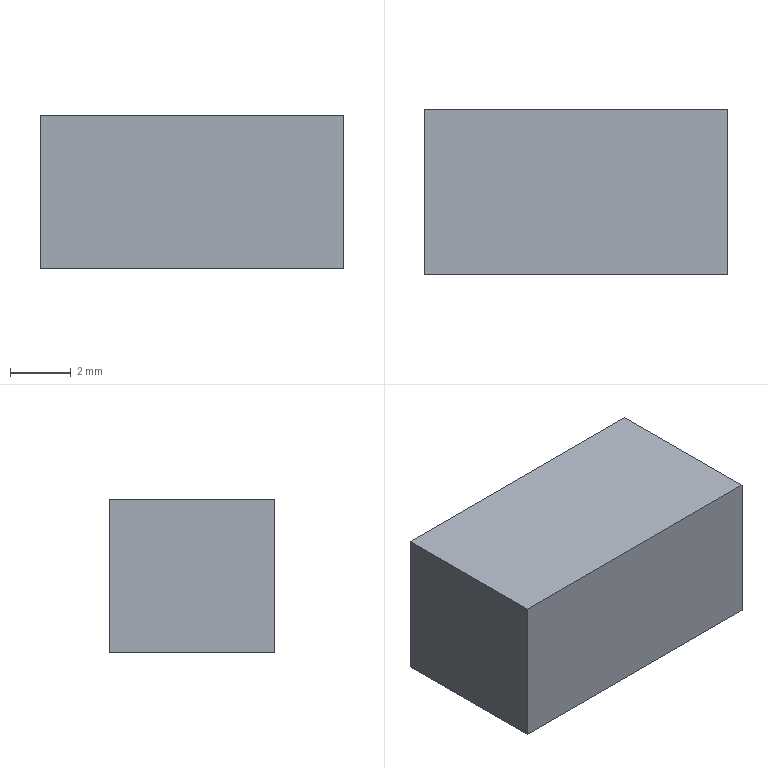Part | NX | features solid 2 | 1 solid | 6 faces | box 10 x 5.446 x 5.048 mm | volume 274.878 mm3 | plane 6
STEP:
#1=CARTESIAN_POINT('',(2250.,364.446,-670.));
#2=VERTEX_POINT('',#1);
#3=CARTESIAN_POINT('',(2250.,359.,-670.));
#4=VERTEX_POINT('',#3);
#5=CARTESIAN_POINT('',(2250.,364.446,-670.));
#6=CARTESIAN_POINT('',(2250.,362.63,-670.));
#7=CARTESIAN_POINT('',(2250.,360.815,-670.));
#8=CARTESIAN_POINT('',(2250.,359.,-670.));
#9=B_SPLINE_CURVE_WITH_KNOTS('',3,(#5,#6,#7,#8),.UNSPECIFIED.,.F.,.F.,(4,4),(0.,0.2595),.PIECEWISE_BEZIER_KNOTS.);
#10=EDGE_CURVE('',#2,#4,#9,.T.);
#11=ORIENTED_EDGE('',*,*,#10,.F.);
#12=CARTESIAN_POINT('',(2260.,364.446,-670.));
#13=VERTEX_POINT('',#12);
#14=CARTESIAN_POINT('',(2260.,364.446,-670.));
#15=DIRECTION('',(-1.,0.,0.));
#16=VECTOR('',#15,1000.);
#17=LINE('',#14,#16);
#18=EDGE_CURVE('',#13,#2,#17,.T.);
#19=ORIENTED_EDGE('',*,*,#18,.F.);
#20=CARTESIAN_POINT('',(2260.,359.,-670.));
#21=VERTEX_POINT('',#20);
#22=CARTESIAN_POINT('',(2260.,364.446,-670.));
#23=CARTESIAN_POINT('',(2260.,362.63,-670.));
#24=CARTESIAN_POINT('',(2260.,360.815,-670.));
#25=CARTESIAN_POINT('',(2260.,359.,-670.));
#26=B_SPLINE_CURVE_WITH_KNOTS('',3,(#22,#23,#24,#25),.UNSPECIFIED.,.F.,.F.,(4,4),(0.,0.2595),.PIECEWISE_BEZIER_KNOTS.);
#27=EDGE_CURVE('',#13,#21,#26,.T.);
#28=ORIENTED_EDGE('',*,*,#27,.T.);
#29=CARTESIAN_POINT('',(2260.,359.,-670.));
#30=DIRECTION('',(-1.,0.,0.));
#31=VECTOR('',#30,1000.);
#32=LINE('',#29,#31);
#33=EDGE_CURVE('',#21,#4,#32,.T.);
#34=ORIENTED_EDGE('',*,*,#33,.T.);
#35=EDGE_LOOP('',(#11,#19,#28,#34));
#36=FACE_BOUND('',#35,.T.);
#37=CARTESIAN_POINT('',(2260.,364.446,-670.));
#38=DIRECTION('',(0.,0.,-1.));
#39=DIRECTION('',(-1.,0.,0.));
#40=AXIS2_PLACEMENT_3D('',#37,#38,#39);
#41=PLANE('',#40);
#42=ADVANCED_FACE('',(#36),#41,.T.);
#43=CARTESIAN_POINT('',(2250.,359.,-664.952));
#44=VERTEX_POINT('',#43);
#45=CARTESIAN_POINT('',(2250.,359.,-670.));
#46=CARTESIAN_POINT('',(2250.,359.,-668.317));
#47=CARTESIAN_POINT('',(2250.,359.,-666.635));
#48=CARTESIAN_POINT('',(2250.,359.,-664.952));
#49=B_SPLINE_CURVE_WITH_KNOTS('',3,(#45,#46,#47,#48),.UNSPECIFIED.,.F.,.F.,(4,4),(0.2595,0.5),.PIECEWISE_BEZIER_KNOTS.);
#50=EDGE_CURVE('',#4,#44,#49,.T.);
#51=ORIENTED_EDGE('',*,*,#50,.F.);
#52=ORIENTED_EDGE('',*,*,#33,.F.);
#53=CARTESIAN_POINT('',(2260.,359.,-664.952));
#54=VERTEX_POINT('',#53);
#55=CARTESIAN_POINT('',(2260.,359.,-670.));
#56=CARTESIAN_POINT('',(2260.,359.,-668.317));
#57=CARTESIAN_POINT('',(2260.,359.,-666.635));
#58=CARTESIAN_POINT('',(2260.,359.,-664.952));
#59=B_SPLINE_CURVE_WITH_KNOTS('',3,(#55,#56,#57,#58),.UNSPECIFIED.,.F.,.F.,(4,4),(0.2595,0.5),.PIECEWISE_BEZIER_KNOTS.);
#60=EDGE_CURVE('',#21,#54,#59,.T.);
#61=ORIENTED_EDGE('',*,*,#60,.T.);
#62=CARTESIAN_POINT('',(2260.,359.,-664.952));
#63=DIRECTION('',(-1.,0.,0.));
#64=VECTOR('',#63,1000.);
#65=LINE('',#62,#64);
#66=EDGE_CURVE('',#54,#44,#65,.T.);
#67=ORIENTED_EDGE('',*,*,#66,.T.);
#68=EDGE_LOOP('',(#51,#52,#61,#67));
#69=FACE_BOUND('',#68,.T.);
#70=CARTESIAN_POINT('',(2260.,359.,-670.));
#71=DIRECTION('',(0.,-1.,0.));
#72=DIRECTION('',(1.,0.,0.));
#73=AXIS2_PLACEMENT_3D('',#70,#71,#72);
#74=PLANE('',#73);
#75=ADVANCED_FACE('',(#69),#74,.T.);
#76=CARTESIAN_POINT('',(2250.,364.446,-664.952));
#77=VERTEX_POINT('',#76);
#78=CARTESIAN_POINT('',(2250.,359.,-664.952));
#79=CARTESIAN_POINT('',(2250.,360.815,-664.952));
#80=CARTESIAN_POINT('',(2250.,362.63,-664.952));
#81=CARTESIAN_POINT('',(2250.,364.446,-664.952));
#82=B_SPLINE_CURVE_WITH_KNOTS('',3,(#78,#79,#80,#81),.UNSPECIFIED.,.F.,.F.,(4,4),(0.5,0.7595),.PIECEWISE_BEZIER_KNOTS.);
#83=EDGE_CURVE('',#44,#77,#82,.T.);
#84=ORIENTED_EDGE('',*,*,#83,.F.);
#85=ORIENTED_EDGE('',*,*,#66,.F.);
#86=CARTESIAN_POINT('',(2260.,364.446,-664.952));
#87=VERTEX_POINT('',#86);
#88=CARTESIAN_POINT('',(2260.,359.,-664.952));
#89=CARTESIAN_POINT('',(2260.,360.815,-664.952));
#90=CARTESIAN_POINT('',(2260.,362.63,-664.952));
#91=CARTESIAN_POINT('',(2260.,364.446,-664.952));
#92=B_SPLINE_CURVE_WITH_KNOTS('',3,(#88,#89,#90,#91),.UNSPECIFIED.,.F.,.F.,(4,4),(0.5,0.7595),.PIECEWISE_BEZIER_KNOTS.);
#93=EDGE_CURVE('',#54,#87,#92,.T.);
#94=ORIENTED_EDGE('',*,*,#93,.T.);
#95=CARTESIAN_POINT('',(2260.,364.446,-664.952));
#96=DIRECTION('',(-1.,0.,0.));
#97=VECTOR('',#96,1000.);
#98=LINE('',#95,#97);
#99=EDGE_CURVE('',#87,#77,#98,.T.);
#100=ORIENTED_EDGE('',*,*,#99,.T.);
#101=EDGE_LOOP('',(#84,#85,#94,#100));
#102=FACE_BOUND('',#101,.T.);
#103=CARTESIAN_POINT('',(2260.,359.,-664.952));
#104=DIRECTION('',(0.,0.,1.));
#105=DIRECTION('',(1.,0.,0.));
#106=AXIS2_PLACEMENT_3D('',#103,#104,#105);
#107=PLANE('',#106);
#108=ADVANCED_FACE('',(#102),#107,.T.);
#109=CARTESIAN_POINT('',(2250.,364.446,-664.952));
#110=CARTESIAN_POINT('',(2250.,364.446,-666.635));
#111=CARTESIAN_POINT('',(2250.,364.446,-668.317));
#112=CARTESIAN_POINT('',(2250.,364.446,-670.));
#113=B_SPLINE_CURVE_WITH_KNOTS('',3,(#109,#110,#111,#112),.UNSPECIFIED.,.F.,.F.,(4,4),(0.7595,1.),.PIECEWISE_BEZIER_KNOTS.);
#114=EDGE_CURVE('',#77,#2,#113,.T.);
#115=ORIENTED_EDGE('',*,*,#114,.F.);
#116=ORIENTED_EDGE('',*,*,#99,.F.);
#117=CARTESIAN_POINT('',(2260.,364.446,-664.952));
#118=CARTESIAN_POINT('',(2260.,364.446,-666.635));
#119=CARTESIAN_POINT('',(2260.,364.446,-668.317));
#120=CARTESIAN_POINT('',(2260.,364.446,-670.));
#121=B_SPLINE_CURVE_WITH_KNOTS('',3,(#117,#118,#119,#120),.UNSPECIFIED.,.F.,.F.,(4,4),(0.7595,1.),.PIECEWISE_BEZIER_KNOTS.);
#122=EDGE_CURVE('',#87,#13,#121,.T.);
#123=ORIENTED_EDGE('',*,*,#122,.T.);
#124=ORIENTED_EDGE('',*,*,#18,.T.);
#125=EDGE_LOOP('',(#115,#116,#123,#124));
#126=FACE_BOUND('',#125,.T.);
#127=CARTESIAN_POINT('',(2260.,364.446,-664.952));
#128=DIRECTION('',(0.,1.,0.));
#129=DIRECTION('',(-1.,0.,0.));
#130=AXIS2_PLACEMENT_3D('',#127,#128,#129);
#131=PLANE('',#130);
#132=ADVANCED_FACE('',(#126),#131,.T.);
#133=ORIENTED_EDGE('',*,*,#27,.F.);
#134=ORIENTED_EDGE('',*,*,#122,.F.);
#135=ORIENTED_EDGE('',*,*,#93,.F.);
#136=ORIENTED_EDGE('',*,*,#60,.F.);
#137=EDGE_LOOP('',(#133,#134,#135,#136));
#138=FACE_BOUND('',#137,.T.);
#139=CARTESIAN_POINT('',(2260.,361.723,-670.));
#140=DIRECTION('',(1.,0.,0.));
#141=DIRECTION('',(0.,1.,0.));
#142=AXIS2_PLACEMENT_3D('',#139,#140,#141);
#143=PLANE('',#142);
#144=ADVANCED_FACE('',(#138),#143,.T.);
#145=ORIENTED_EDGE('',*,*,#10,.T.);
#146=ORIENTED_EDGE('',*,*,#50,.T.);
#147=ORIENTED_EDGE('',*,*,#83,.T.);
#148=ORIENTED_EDGE('',*,*,#114,.T.);
#149=EDGE_LOOP('',(#145,#146,#147,#148));
#150=FACE_BOUND('',#149,.T.);
#151=CARTESIAN_POINT('',(2250.,361.723,-670.));
#152=DIRECTION('',(1.,0.,0.));
#153=DIRECTION('',(0.,1.,0.));
#154=AXIS2_PLACEMENT_3D('',#151,#152,#153);
#155=PLANE('',#154);
#156=ADVANCED_FACE('',(#150),#155,.F.);
#157=CLOSED_SHELL('',(#42,#75,#108,#132,#144,#156));
#158=MANIFOLD_SOLID_BREP('',#157);
#159=(LENGTH_UNIT()NAMED_UNIT(*)SI_UNIT(.MILLI.,.METRE.));
#160=UNCERTAINTY_MEASURE_WITH_UNIT(LENGTH_MEASURE(0.00001),#159,'','');
#161=(NAMED_UNIT(*)PLANE_ANGLE_UNIT()SI_UNIT($,.RADIAN.));
#162=(NAMED_UNIT(*)SI_UNIT($,.STERADIAN.)SOLID_ANGLE_UNIT());
#163=(GEOMETRIC_REPRESENTATION_CONTEXT(3)GLOBAL_UNCERTAINTY_ASSIGNED_CONTEXT((#160))GLOBAL_UNIT_ASSIGNED_CONTEXT((#159,#161,#162))REPRESENTATION_CONTEXT('',''));
#164=ADVANCED_BREP_SHAPE_REPRESENTATION('',(#158),#163);